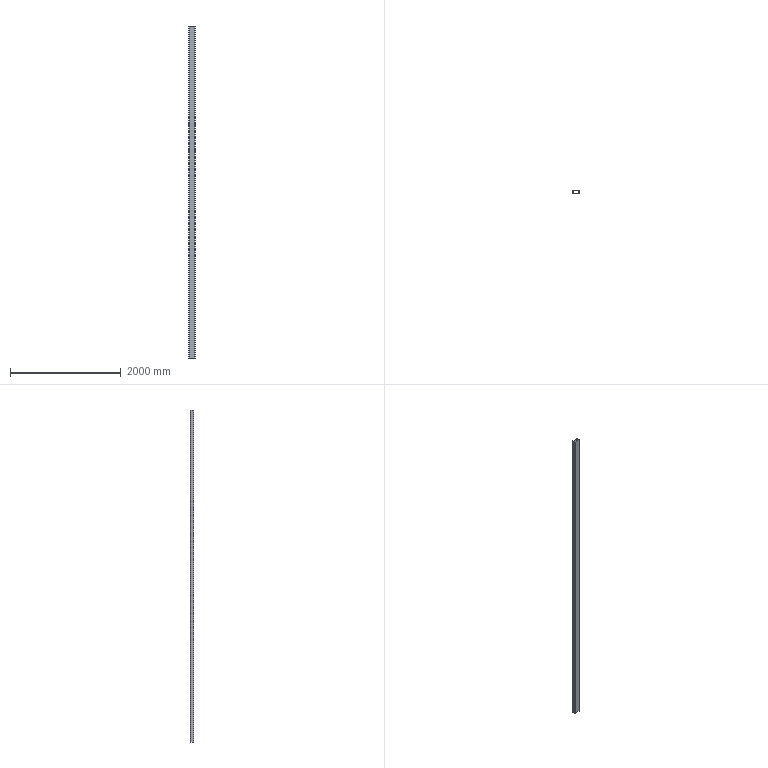Part | SolidWorks | features Extrusion 1 | 1 solid | 18 faces | box 120 x 60 x 6000 mm | volume 9813717 mm3 | plane 10 | cylinder 8 | commonest cylinder face diameters 10 x4 20 x4
STEP:
#1=CARTESIAN_POINT('',(110.,0.,6000.));
#2=VERTEX_POINT('',#1);
#3=CARTESIAN_POINT('',(120.,10.,6000.));
#4=VERTEX_POINT('',#3);
#5=CARTESIAN_POINT('',(110.,10.,6000.));
#6=DIRECTION('',(0.,0.,1.));
#7=DIRECTION('',(-1.,0.,0.));
#8=AXIS2_PLACEMENT_3D('',#5,#6,#7);
#9=CIRCLE('',#8,10.);
#10=EDGE_CURVE('',#2,#4,#9,.T.);
#11=ORIENTED_EDGE('',*,*,#10,.T.);
#12=CARTESIAN_POINT('',(120.,50.,6000.));
#13=VERTEX_POINT('',#12);
#14=CARTESIAN_POINT('',(120.,10.,6000.));
#15=DIRECTION('',(0.,1.,0.));
#16=VECTOR('',#15,1000.);
#17=LINE('',#14,#16);
#18=EDGE_CURVE('',#4,#13,#17,.T.);
#19=ORIENTED_EDGE('',*,*,#18,.T.);
#20=CARTESIAN_POINT('',(110.,60.,6000.));
#21=VERTEX_POINT('',#20);
#22=CARTESIAN_POINT('',(110.,50.,6000.));
#23=DIRECTION('',(0.,0.,1.));
#24=DIRECTION('',(1.,0.,0.));
#25=AXIS2_PLACEMENT_3D('',#22,#23,#24);
#26=CIRCLE('',#25,10.);
#27=EDGE_CURVE('',#13,#21,#26,.T.);
#28=ORIENTED_EDGE('',*,*,#27,.T.);
#29=CARTESIAN_POINT('',(10.,60.,6000.));
#30=VERTEX_POINT('',#29);
#31=CARTESIAN_POINT('',(10.,60.,6000.));
#32=DIRECTION('',(-1.,0.,0.));
#33=VECTOR('',#32,1000.);
#34=LINE('',#31,#33);
#35=EDGE_CURVE('',#21,#30,#34,.T.);
#36=ORIENTED_EDGE('',*,*,#35,.T.);
#37=CARTESIAN_POINT('',(0.,50.,6000.));
#38=VERTEX_POINT('',#37);
#39=CARTESIAN_POINT('',(10.,50.,6000.));
#40=DIRECTION('',(0.,0.,1.));
#41=DIRECTION('',(-1.,0.,0.));
#42=AXIS2_PLACEMENT_3D('',#39,#40,#41);
#43=CIRCLE('',#42,10.);
#44=EDGE_CURVE('',#30,#38,#43,.T.);
#45=ORIENTED_EDGE('',*,*,#44,.T.);
#46=CARTESIAN_POINT('',(0.,10.,6000.));
#47=VERTEX_POINT('',#46);
#48=CARTESIAN_POINT('',(0.,10.,6000.));
#49=DIRECTION('',(0.,-1.,0.));
#50=VECTOR('',#49,1000.);
#51=LINE('',#48,#50);
#52=EDGE_CURVE('',#38,#47,#51,.T.);
#53=ORIENTED_EDGE('',*,*,#52,.T.);
#54=CARTESIAN_POINT('',(10.,0.,6000.));
#55=VERTEX_POINT('',#54);
#56=CARTESIAN_POINT('',(10.,10.,6000.));
#57=DIRECTION('',(0.,0.,1.));
#58=DIRECTION('',(-1.,0.,0.));
#59=AXIS2_PLACEMENT_3D('',#56,#57,#58);
#60=CIRCLE('',#59,10.);
#61=EDGE_CURVE('',#47,#55,#60,.T.);
#62=ORIENTED_EDGE('',*,*,#61,.T.);
#63=CARTESIAN_POINT('',(10.,0.,6000.));
#64=DIRECTION('',(1.,0.,0.));
#65=VECTOR('',#64,1000.);
#66=LINE('',#63,#65);
#67=EDGE_CURVE('',#55,#2,#66,.T.);
#68=ORIENTED_EDGE('',*,*,#67,.T.);
#69=EDGE_LOOP('',(#11,#19,#28,#36,#45,#53,#62,#68));
#70=FACE_OUTER_BOUND('',#69,.T.);
#71=CARTESIAN_POINT('',(10.,55.,6000.));
#72=VERTEX_POINT('',#71);
#73=CARTESIAN_POINT('',(5.,50.,6000.));
#74=VERTEX_POINT('',#73);
#75=CARTESIAN_POINT('',(10.,50.,6000.));
#76=DIRECTION('',(0.,0.,1.));
#77=DIRECTION('',(-1.,0.,0.));
#78=AXIS2_PLACEMENT_3D('',#75,#76,#77);
#79=CIRCLE('',#78,5.);
#80=EDGE_CURVE('',#72,#74,#79,.T.);
#81=ORIENTED_EDGE('',*,*,#80,.F.);
#82=CARTESIAN_POINT('',(110.,55.,6000.));
#83=VERTEX_POINT('',#82);
#84=CARTESIAN_POINT('',(10.,55.,6000.));
#85=DIRECTION('',(-1.,0.,0.));
#86=VECTOR('',#85,1000.);
#87=LINE('',#84,#86);
#88=EDGE_CURVE('',#83,#72,#87,.T.);
#89=ORIENTED_EDGE('',*,*,#88,.F.);
#90=CARTESIAN_POINT('',(115.,50.,6000.));
#91=VERTEX_POINT('',#90);
#92=CARTESIAN_POINT('',(110.,50.,6000.));
#93=DIRECTION('',(0.,0.,1.));
#94=DIRECTION('',(1.,0.,0.));
#95=AXIS2_PLACEMENT_3D('',#92,#93,#94);
#96=CIRCLE('',#95,5.);
#97=EDGE_CURVE('',#91,#83,#96,.T.);
#98=ORIENTED_EDGE('',*,*,#97,.F.);
#99=CARTESIAN_POINT('',(115.,10.,6000.));
#100=VERTEX_POINT('',#99);
#101=CARTESIAN_POINT('',(115.,10.,6000.));
#102=DIRECTION('',(0.,1.,0.));
#103=VECTOR('',#102,1000.);
#104=LINE('',#101,#103);
#105=EDGE_CURVE('',#100,#91,#104,.T.);
#106=ORIENTED_EDGE('',*,*,#105,.F.);
#107=CARTESIAN_POINT('',(110.,5.,6000.));
#108=VERTEX_POINT('',#107);
#109=CARTESIAN_POINT('',(110.,10.,6000.));
#110=DIRECTION('',(0.,0.,1.));
#111=DIRECTION('',(-1.,0.,0.));
#112=AXIS2_PLACEMENT_3D('',#109,#110,#111);
#113=CIRCLE('',#112,5.);
#114=EDGE_CURVE('',#108,#100,#113,.T.);
#115=ORIENTED_EDGE('',*,*,#114,.F.);
#116=CARTESIAN_POINT('',(10.,5.,6000.));
#117=VERTEX_POINT('',#116);
#118=CARTESIAN_POINT('',(10.,5.,6000.));
#119=DIRECTION('',(1.,0.,0.));
#120=VECTOR('',#119,1000.);
#121=LINE('',#118,#120);
#122=EDGE_CURVE('',#117,#108,#121,.T.);
#123=ORIENTED_EDGE('',*,*,#122,.F.);
#124=CARTESIAN_POINT('',(5.,10.,6000.));
#125=VERTEX_POINT('',#124);
#126=CARTESIAN_POINT('',(10.,10.,6000.));
#127=DIRECTION('',(0.,0.,1.));
#128=DIRECTION('',(-1.,0.,0.));
#129=AXIS2_PLACEMENT_3D('',#126,#127,#128);
#130=CIRCLE('',#129,5.);
#131=EDGE_CURVE('',#125,#117,#130,.T.);
#132=ORIENTED_EDGE('',*,*,#131,.F.);
#133=CARTESIAN_POINT('',(5.,10.,6000.));
#134=DIRECTION('',(0.,-1.,0.));
#135=VECTOR('',#134,1000.);
#136=LINE('',#133,#135);
#137=EDGE_CURVE('',#74,#125,#136,.T.);
#138=ORIENTED_EDGE('',*,*,#137,.F.);
#139=EDGE_LOOP('',(#81,#89,#98,#106,#115,#123,#132,#138));
#140=FACE_BOUND('',#139,.T.);
#141=CARTESIAN_POINT('',(110.,10.,6000.));
#142=DIRECTION('',(0.,0.,-1.));
#143=DIRECTION('',(-1.,0.,0.));
#144=AXIS2_PLACEMENT_3D('',#141,#142,#143);
#145=PLANE('',#144);
#146=ADVANCED_FACE('',(#70,#140),#145,.F.);
#147=CARTESIAN_POINT('',(110.,0.,0.));
#148=VERTEX_POINT('',#147);
#149=CARTESIAN_POINT('',(120.,10.,0.));
#150=VERTEX_POINT('',#149);
#151=CARTESIAN_POINT('',(110.,10.,0.));
#152=DIRECTION('',(0.,0.,1.));
#153=DIRECTION('',(-1.,0.,0.));
#154=AXIS2_PLACEMENT_3D('',#151,#152,#153);
#155=CIRCLE('',#154,10.);
#156=EDGE_CURVE('',#148,#150,#155,.T.);
#157=ORIENTED_EDGE('',*,*,#156,.F.);
#158=CARTESIAN_POINT('',(10.,0.,0.));
#159=VERTEX_POINT('',#158);
#160=CARTESIAN_POINT('',(10.,0.,0.));
#161=DIRECTION('',(1.,0.,0.));
#162=VECTOR('',#161,1000.);
#163=LINE('',#160,#162);
#164=EDGE_CURVE('',#159,#148,#163,.T.);
#165=ORIENTED_EDGE('',*,*,#164,.F.);
#166=CARTESIAN_POINT('',(0.,10.,0.));
#167=VERTEX_POINT('',#166);
#168=CARTESIAN_POINT('',(10.,10.,0.));
#169=DIRECTION('',(0.,0.,1.));
#170=DIRECTION('',(-1.,0.,0.));
#171=AXIS2_PLACEMENT_3D('',#168,#169,#170);
#172=CIRCLE('',#171,10.);
#173=EDGE_CURVE('',#167,#159,#172,.T.);
#174=ORIENTED_EDGE('',*,*,#173,.F.);
#175=CARTESIAN_POINT('',(0.,50.,0.));
#176=VERTEX_POINT('',#175);
#177=CARTESIAN_POINT('',(0.,10.,0.));
#178=DIRECTION('',(0.,-1.,0.));
#179=VECTOR('',#178,1000.);
#180=LINE('',#177,#179);
#181=EDGE_CURVE('',#176,#167,#180,.T.);
#182=ORIENTED_EDGE('',*,*,#181,.F.);
#183=CARTESIAN_POINT('',(10.,60.,0.));
#184=VERTEX_POINT('',#183);
#185=CARTESIAN_POINT('',(10.,50.,0.));
#186=DIRECTION('',(0.,0.,1.));
#187=DIRECTION('',(-1.,0.,0.));
#188=AXIS2_PLACEMENT_3D('',#185,#186,#187);
#189=CIRCLE('',#188,10.);
#190=EDGE_CURVE('',#184,#176,#189,.T.);
#191=ORIENTED_EDGE('',*,*,#190,.F.);
#192=CARTESIAN_POINT('',(110.,60.,0.));
#193=VERTEX_POINT('',#192);
#194=CARTESIAN_POINT('',(10.,60.,0.));
#195=DIRECTION('',(-1.,0.,0.));
#196=VECTOR('',#195,1000.);
#197=LINE('',#194,#196);
#198=EDGE_CURVE('',#193,#184,#197,.T.);
#199=ORIENTED_EDGE('',*,*,#198,.F.);
#200=CARTESIAN_POINT('',(120.,50.,0.));
#201=VERTEX_POINT('',#200);
#202=CARTESIAN_POINT('',(110.,50.,0.));
#203=DIRECTION('',(0.,0.,1.));
#204=DIRECTION('',(1.,0.,0.));
#205=AXIS2_PLACEMENT_3D('',#202,#203,#204);
#206=CIRCLE('',#205,10.);
#207=EDGE_CURVE('',#201,#193,#206,.T.);
#208=ORIENTED_EDGE('',*,*,#207,.F.);
#209=CARTESIAN_POINT('',(120.,10.,0.));
#210=DIRECTION('',(0.,1.,0.));
#211=VECTOR('',#210,1000.);
#212=LINE('',#209,#211);
#213=EDGE_CURVE('',#150,#201,#212,.T.);
#214=ORIENTED_EDGE('',*,*,#213,.F.);
#215=EDGE_LOOP('',(#157,#165,#174,#182,#191,#199,#208,#214));
#216=FACE_OUTER_BOUND('',#215,.T.);
#217=CARTESIAN_POINT('',(110.,55.,0.));
#218=VERTEX_POINT('',#217);
#219=CARTESIAN_POINT('',(10.,55.,0.));
#220=VERTEX_POINT('',#219);
#221=CARTESIAN_POINT('',(10.,55.,0.));
#222=DIRECTION('',(-1.,0.,0.));
#223=VECTOR('',#222,1000.);
#224=LINE('',#221,#223);
#225=EDGE_CURVE('',#218,#220,#224,.T.);
#226=ORIENTED_EDGE('',*,*,#225,.T.);
#227=CARTESIAN_POINT('',(5.,50.,0.));
#228=VERTEX_POINT('',#227);
#229=CARTESIAN_POINT('',(10.,50.,0.));
#230=DIRECTION('',(0.,0.,1.));
#231=DIRECTION('',(-1.,0.,0.));
#232=AXIS2_PLACEMENT_3D('',#229,#230,#231);
#233=CIRCLE('',#232,5.);
#234=EDGE_CURVE('',#220,#228,#233,.T.);
#235=ORIENTED_EDGE('',*,*,#234,.T.);
#236=CARTESIAN_POINT('',(5.,10.,0.));
#237=VERTEX_POINT('',#236);
#238=CARTESIAN_POINT('',(5.,10.,0.));
#239=DIRECTION('',(0.,-1.,0.));
#240=VECTOR('',#239,1000.);
#241=LINE('',#238,#240);
#242=EDGE_CURVE('',#228,#237,#241,.T.);
#243=ORIENTED_EDGE('',*,*,#242,.T.);
#244=CARTESIAN_POINT('',(10.,5.,0.));
#245=VERTEX_POINT('',#244);
#246=CARTESIAN_POINT('',(10.,10.,0.));
#247=DIRECTION('',(0.,0.,1.));
#248=DIRECTION('',(-1.,0.,0.));
#249=AXIS2_PLACEMENT_3D('',#246,#247,#248);
#250=CIRCLE('',#249,5.);
#251=EDGE_CURVE('',#237,#245,#250,.T.);
#252=ORIENTED_EDGE('',*,*,#251,.T.);
#253=CARTESIAN_POINT('',(110.,5.,0.));
#254=VERTEX_POINT('',#253);
#255=CARTESIAN_POINT('',(10.,5.,0.));
#256=DIRECTION('',(1.,0.,0.));
#257=VECTOR('',#256,1000.);
#258=LINE('',#255,#257);
#259=EDGE_CURVE('',#245,#254,#258,.T.);
#260=ORIENTED_EDGE('',*,*,#259,.T.);
#261=CARTESIAN_POINT('',(115.,10.,0.));
#262=VERTEX_POINT('',#261);
#263=CARTESIAN_POINT('',(110.,10.,0.));
#264=DIRECTION('',(0.,0.,1.));
#265=DIRECTION('',(-1.,0.,0.));
#266=AXIS2_PLACEMENT_3D('',#263,#264,#265);
#267=CIRCLE('',#266,5.);
#268=EDGE_CURVE('',#254,#262,#267,.T.);
#269=ORIENTED_EDGE('',*,*,#268,.T.);
#270=CARTESIAN_POINT('',(115.,50.,0.));
#271=VERTEX_POINT('',#270);
#272=CARTESIAN_POINT('',(115.,10.,0.));
#273=DIRECTION('',(0.,1.,0.));
#274=VECTOR('',#273,1000.);
#275=LINE('',#272,#274);
#276=EDGE_CURVE('',#262,#271,#275,.T.);
#277=ORIENTED_EDGE('',*,*,#276,.T.);
#278=CARTESIAN_POINT('',(110.,50.,0.));
#279=DIRECTION('',(0.,0.,1.));
#280=DIRECTION('',(1.,0.,0.));
#281=AXIS2_PLACEMENT_3D('',#278,#279,#280);
#282=CIRCLE('',#281,5.);
#283=EDGE_CURVE('',#271,#218,#282,.T.);
#284=ORIENTED_EDGE('',*,*,#283,.T.);
#285=EDGE_LOOP('',(#226,#235,#243,#252,#260,#269,#277,#284));
#286=FACE_BOUND('',#285,.T.);
#287=CARTESIAN_POINT('',(110.,10.,0.));
#288=DIRECTION('',(0.,0.,-1.));
#289=DIRECTION('',(-1.,0.,0.));
#290=AXIS2_PLACEMENT_3D('',#287,#288,#289);
#291=PLANE('',#290);
#292=ADVANCED_FACE('',(#216,#286),#291,.T.);
#293=ORIENTED_EDGE('',*,*,#156,.T.);
#294=CARTESIAN_POINT('',(120.,10.,6000.));
#295=DIRECTION('',(0.,0.,-1.));
#296=VECTOR('',#295,1000.);
#297=LINE('',#294,#296);
#298=EDGE_CURVE('',#4,#150,#297,.T.);
#299=ORIENTED_EDGE('',*,*,#298,.F.);
#300=ORIENTED_EDGE('',*,*,#10,.F.);
#301=CARTESIAN_POINT('',(110.,0.,6000.));
#302=DIRECTION('',(0.,0.,-1.));
#303=VECTOR('',#302,1000.);
#304=LINE('',#301,#303);
#305=EDGE_CURVE('',#2,#148,#304,.T.);
#306=ORIENTED_EDGE('',*,*,#305,.T.);
#307=EDGE_LOOP('',(#293,#299,#300,#306));
#308=FACE_OUTER_BOUND('',#307,.T.);
#309=CARTESIAN_POINT('',(110.,10.,6000.));
#310=DIRECTION('',(0.,0.,-1.));
#311=DIRECTION('',(-1.,0.,0.));
#312=AXIS2_PLACEMENT_3D('',#309,#310,#311);
#313=CYLINDRICAL_SURFACE('',#312,10.);
#314=ADVANCED_FACE('',(#308),#313,.T.);
#315=ORIENTED_EDGE('',*,*,#213,.T.);
#316=CARTESIAN_POINT('',(120.,50.,6000.));
#317=DIRECTION('',(0.,0.,-1.));
#318=VECTOR('',#317,1000.);
#319=LINE('',#316,#318);
#320=EDGE_CURVE('',#13,#201,#319,.T.);
#321=ORIENTED_EDGE('',*,*,#320,.F.);
#322=ORIENTED_EDGE('',*,*,#18,.F.);
#323=ORIENTED_EDGE('',*,*,#298,.T.);
#324=EDGE_LOOP('',(#315,#321,#322,#323));
#325=FACE_OUTER_BOUND('',#324,.T.);
#326=CARTESIAN_POINT('',(120.,10.,6000.));
#327=DIRECTION('',(-1.,0.,0.));
#328=DIRECTION('',(0.,-1.,0.));
#329=AXIS2_PLACEMENT_3D('',#326,#327,#328);
#330=PLANE('',#329);
#331=ADVANCED_FACE('',(#325),#330,.F.);
#332=ORIENTED_EDGE('',*,*,#207,.T.);
#333=CARTESIAN_POINT('',(110.,60.,6000.));
#334=DIRECTION('',(0.,0.,-1.));
#335=VECTOR('',#334,1000.);
#336=LINE('',#333,#335);
#337=EDGE_CURVE('',#21,#193,#336,.T.);
#338=ORIENTED_EDGE('',*,*,#337,.F.);
#339=ORIENTED_EDGE('',*,*,#27,.F.);
#340=ORIENTED_EDGE('',*,*,#320,.T.);
#341=EDGE_LOOP('',(#332,#338,#339,#340));
#342=FACE_OUTER_BOUND('',#341,.T.);
#343=CARTESIAN_POINT('',(110.,50.,6000.));
#344=DIRECTION('',(0.,0.,-1.));
#345=DIRECTION('',(-1.,0.,0.));
#346=AXIS2_PLACEMENT_3D('',#343,#344,#345);
#347=CYLINDRICAL_SURFACE('',#346,10.);
#348=ADVANCED_FACE('',(#342),#347,.T.);
#349=ORIENTED_EDGE('',*,*,#198,.T.);
#350=CARTESIAN_POINT('',(10.,60.,6000.));
#351=DIRECTION('',(0.,0.,-1.));
#352=VECTOR('',#351,1000.);
#353=LINE('',#350,#352);
#354=EDGE_CURVE('',#30,#184,#353,.T.);
#355=ORIENTED_EDGE('',*,*,#354,.F.);
#356=ORIENTED_EDGE('',*,*,#35,.F.);
#357=ORIENTED_EDGE('',*,*,#337,.T.);
#358=EDGE_LOOP('',(#349,#355,#356,#357));
#359=FACE_OUTER_BOUND('',#358,.T.);
#360=CARTESIAN_POINT('',(10.,60.,6000.));
#361=DIRECTION('',(0.,-1.,0.));
#362=DIRECTION('',(0.,0.,-1.));
#363=AXIS2_PLACEMENT_3D('',#360,#361,#362);
#364=PLANE('',#363);
#365=ADVANCED_FACE('',(#359),#364,.F.);
#366=ORIENTED_EDGE('',*,*,#190,.T.);
#367=CARTESIAN_POINT('',(0.,50.,6000.));
#368=DIRECTION('',(0.,0.,-1.));
#369=VECTOR('',#368,1000.);
#370=LINE('',#367,#369);
#371=EDGE_CURVE('',#38,#176,#370,.T.);
#372=ORIENTED_EDGE('',*,*,#371,.F.);
#373=ORIENTED_EDGE('',*,*,#44,.F.);
#374=ORIENTED_EDGE('',*,*,#354,.T.);
#375=EDGE_LOOP('',(#366,#372,#373,#374));
#376=FACE_OUTER_BOUND('',#375,.T.);
#377=CARTESIAN_POINT('',(10.,50.,6000.));
#378=DIRECTION('',(0.,0.,-1.));
#379=DIRECTION('',(-1.,0.,0.));
#380=AXIS2_PLACEMENT_3D('',#377,#378,#379);
#381=CYLINDRICAL_SURFACE('',#380,10.);
#382=ADVANCED_FACE('',(#376),#381,.T.);
#383=ORIENTED_EDGE('',*,*,#181,.T.);
#384=CARTESIAN_POINT('',(0.,10.,6000.));
#385=DIRECTION('',(0.,0.,-1.));
#386=VECTOR('',#385,1000.);
#387=LINE('',#384,#386);
#388=EDGE_CURVE('',#47,#167,#387,.T.);
#389=ORIENTED_EDGE('',*,*,#388,.F.);
#390=ORIENTED_EDGE('',*,*,#52,.F.);
#391=ORIENTED_EDGE('',*,*,#371,.T.);
#392=EDGE_LOOP('',(#383,#389,#390,#391));
#393=FACE_OUTER_BOUND('',#392,.T.);
#394=CARTESIAN_POINT('',(0.,10.,6000.));
#395=DIRECTION('',(1.,0.,0.));
#396=DIRECTION('',(0.,1.,0.));
#397=AXIS2_PLACEMENT_3D('',#394,#395,#396);
#398=PLANE('',#397);
#399=ADVANCED_FACE('',(#393),#398,.F.);
#400=ORIENTED_EDGE('',*,*,#173,.T.);
#401=CARTESIAN_POINT('',(10.,0.,6000.));
#402=DIRECTION('',(0.,0.,-1.));
#403=VECTOR('',#402,1000.);
#404=LINE('',#401,#403);
#405=EDGE_CURVE('',#55,#159,#404,.T.);
#406=ORIENTED_EDGE('',*,*,#405,.F.);
#407=ORIENTED_EDGE('',*,*,#61,.F.);
#408=ORIENTED_EDGE('',*,*,#388,.T.);
#409=EDGE_LOOP('',(#400,#406,#407,#408));
#410=FACE_OUTER_BOUND('',#409,.T.);
#411=CARTESIAN_POINT('',(10.,10.,6000.));
#412=DIRECTION('',(0.,0.,-1.));
#413=DIRECTION('',(-1.,0.,0.));
#414=AXIS2_PLACEMENT_3D('',#411,#412,#413);
#415=CYLINDRICAL_SURFACE('',#414,10.);
#416=ADVANCED_FACE('',(#410),#415,.T.);
#417=ORIENTED_EDGE('',*,*,#164,.T.);
#418=ORIENTED_EDGE('',*,*,#305,.F.);
#419=ORIENTED_EDGE('',*,*,#67,.F.);
#420=ORIENTED_EDGE('',*,*,#405,.T.);
#421=EDGE_LOOP('',(#417,#418,#419,#420));
#422=FACE_OUTER_BOUND('',#421,.T.);
#423=CARTESIAN_POINT('',(10.,0.,6000.));
#424=DIRECTION('',(0.,1.,0.));
#425=DIRECTION('',(0.,0.,1.));
#426=AXIS2_PLACEMENT_3D('',#423,#424,#425);
#427=PLANE('',#426);
#428=ADVANCED_FACE('',(#422),#427,.F.);
#429=ORIENTED_EDGE('',*,*,#234,.F.);
#430=CARTESIAN_POINT('',(10.,55.,6000.));
#431=DIRECTION('',(0.,0.,-1.));
#432=VECTOR('',#431,1000.);
#433=LINE('',#430,#432);
#434=EDGE_CURVE('',#72,#220,#433,.T.);
#435=ORIENTED_EDGE('',*,*,#434,.F.);
#436=ORIENTED_EDGE('',*,*,#80,.T.);
#437=CARTESIAN_POINT('',(5.,50.,6000.));
#438=DIRECTION('',(0.,0.,-1.));
#439=VECTOR('',#438,1000.);
#440=LINE('',#437,#439);
#441=EDGE_CURVE('',#74,#228,#440,.T.);
#442=ORIENTED_EDGE('',*,*,#441,.T.);
#443=EDGE_LOOP('',(#429,#435,#436,#442));
#444=FACE_OUTER_BOUND('',#443,.T.);
#445=CARTESIAN_POINT('',(10.,50.,6000.));
#446=DIRECTION('',(0.,0.,-1.));
#447=DIRECTION('',(-1.,0.,0.));
#448=AXIS2_PLACEMENT_3D('',#445,#446,#447);
#449=CYLINDRICAL_SURFACE('',#448,5.);
#450=ADVANCED_FACE('',(#444),#449,.F.);
#451=ORIENTED_EDGE('',*,*,#242,.F.);
#452=ORIENTED_EDGE('',*,*,#441,.F.);
#453=ORIENTED_EDGE('',*,*,#137,.T.);
#454=CARTESIAN_POINT('',(5.,10.,6000.));
#455=DIRECTION('',(0.,0.,-1.));
#456=VECTOR('',#455,1000.);
#457=LINE('',#454,#456);
#458=EDGE_CURVE('',#125,#237,#457,.T.);
#459=ORIENTED_EDGE('',*,*,#458,.T.);
#460=EDGE_LOOP('',(#451,#452,#453,#459));
#461=FACE_OUTER_BOUND('',#460,.T.);
#462=CARTESIAN_POINT('',(5.,10.,6000.));
#463=DIRECTION('',(1.,0.,0.));
#464=DIRECTION('',(0.,1.,0.));
#465=AXIS2_PLACEMENT_3D('',#462,#463,#464);
#466=PLANE('',#465);
#467=ADVANCED_FACE('',(#461),#466,.T.);
#468=ORIENTED_EDGE('',*,*,#251,.F.);
#469=ORIENTED_EDGE('',*,*,#458,.F.);
#470=ORIENTED_EDGE('',*,*,#131,.T.);
#471=CARTESIAN_POINT('',(10.,5.,6000.));
#472=DIRECTION('',(0.,0.,-1.));
#473=VECTOR('',#472,1000.);
#474=LINE('',#471,#473);
#475=EDGE_CURVE('',#117,#245,#474,.T.);
#476=ORIENTED_EDGE('',*,*,#475,.T.);
#477=EDGE_LOOP('',(#468,#469,#470,#476));
#478=FACE_OUTER_BOUND('',#477,.T.);
#479=CARTESIAN_POINT('',(10.,10.,6000.));
#480=DIRECTION('',(0.,0.,-1.));
#481=DIRECTION('',(-1.,0.,0.));
#482=AXIS2_PLACEMENT_3D('',#479,#480,#481);
#483=CYLINDRICAL_SURFACE('',#482,5.);
#484=ADVANCED_FACE('',(#478),#483,.F.);
#485=ORIENTED_EDGE('',*,*,#259,.F.);
#486=ORIENTED_EDGE('',*,*,#475,.F.);
#487=ORIENTED_EDGE('',*,*,#122,.T.);
#488=CARTESIAN_POINT('',(110.,5.,6000.));
#489=DIRECTION('',(0.,0.,-1.));
#490=VECTOR('',#489,1000.);
#491=LINE('',#488,#490);
#492=EDGE_CURVE('',#108,#254,#491,.T.);
#493=ORIENTED_EDGE('',*,*,#492,.T.);
#494=EDGE_LOOP('',(#485,#486,#487,#493));
#495=FACE_OUTER_BOUND('',#494,.T.);
#496=CARTESIAN_POINT('',(10.,5.,6000.));
#497=DIRECTION('',(0.,1.,0.));
#498=DIRECTION('',(0.,0.,1.));
#499=AXIS2_PLACEMENT_3D('',#496,#497,#498);
#500=PLANE('',#499);
#501=ADVANCED_FACE('',(#495),#500,.T.);
#502=ORIENTED_EDGE('',*,*,#268,.F.);
#503=ORIENTED_EDGE('',*,*,#492,.F.);
#504=ORIENTED_EDGE('',*,*,#114,.T.);
#505=CARTESIAN_POINT('',(115.,10.,6000.));
#506=DIRECTION('',(0.,0.,-1.));
#507=VECTOR('',#506,1000.);
#508=LINE('',#505,#507);
#509=EDGE_CURVE('',#100,#262,#508,.T.);
#510=ORIENTED_EDGE('',*,*,#509,.T.);
#511=EDGE_LOOP('',(#502,#503,#504,#510));
#512=FACE_OUTER_BOUND('',#511,.T.);
#513=CARTESIAN_POINT('',(110.,10.,6000.));
#514=DIRECTION('',(0.,0.,-1.));
#515=DIRECTION('',(-1.,0.,0.));
#516=AXIS2_PLACEMENT_3D('',#513,#514,#515);
#517=CYLINDRICAL_SURFACE('',#516,5.);
#518=ADVANCED_FACE('',(#512),#517,.F.);
#519=ORIENTED_EDGE('',*,*,#276,.F.);
#520=ORIENTED_EDGE('',*,*,#509,.F.);
#521=ORIENTED_EDGE('',*,*,#105,.T.);
#522=CARTESIAN_POINT('',(115.,50.,6000.));
#523=DIRECTION('',(0.,0.,-1.));
#524=VECTOR('',#523,1000.);
#525=LINE('',#522,#524);
#526=EDGE_CURVE('',#91,#271,#525,.T.);
#527=ORIENTED_EDGE('',*,*,#526,.T.);
#528=EDGE_LOOP('',(#519,#520,#521,#527));
#529=FACE_OUTER_BOUND('',#528,.T.);
#530=CARTESIAN_POINT('',(115.,10.,6000.));
#531=DIRECTION('',(-1.,0.,0.));
#532=DIRECTION('',(0.,0.,1.));
#533=AXIS2_PLACEMENT_3D('',#530,#531,#532);
#534=PLANE('',#533);
#535=ADVANCED_FACE('',(#529),#534,.T.);
#536=ORIENTED_EDGE('',*,*,#283,.F.);
#537=ORIENTED_EDGE('',*,*,#526,.F.);
#538=ORIENTED_EDGE('',*,*,#97,.T.);
#539=CARTESIAN_POINT('',(110.,55.,6000.));
#540=DIRECTION('',(0.,0.,-1.));
#541=VECTOR('',#540,1000.);
#542=LINE('',#539,#541);
#543=EDGE_CURVE('',#83,#218,#542,.T.);
#544=ORIENTED_EDGE('',*,*,#543,.T.);
#545=EDGE_LOOP('',(#536,#537,#538,#544));
#546=FACE_OUTER_BOUND('',#545,.T.);
#547=CARTESIAN_POINT('',(110.,50.,6000.));
#548=DIRECTION('',(0.,0.,-1.));
#549=DIRECTION('',(-1.,0.,0.));
#550=AXIS2_PLACEMENT_3D('',#547,#548,#549);
#551=CYLINDRICAL_SURFACE('',#550,5.);
#552=ADVANCED_FACE('',(#546),#551,.F.);
#553=ORIENTED_EDGE('',*,*,#225,.F.);
#554=ORIENTED_EDGE('',*,*,#543,.F.);
#555=ORIENTED_EDGE('',*,*,#88,.T.);
#556=ORIENTED_EDGE('',*,*,#434,.T.);
#557=EDGE_LOOP('',(#553,#554,#555,#556));
#558=FACE_OUTER_BOUND('',#557,.T.);
#559=CARTESIAN_POINT('',(10.,55.,6000.));
#560=DIRECTION('',(0.,-1.,0.));
#561=DIRECTION('',(0.,0.,-1.));
#562=AXIS2_PLACEMENT_3D('',#559,#560,#561);
#563=PLANE('',#562);
#564=ADVANCED_FACE('',(#558),#563,.T.);
#565=CLOSED_SHELL('',(#146,#292,#314,#331,#348,#365,#382,#399,#416,#428,#450,#467,#484,#501,#518,#535,#552,#564));
#566=MANIFOLD_SOLID_BREP('',#565);
#567=CARTESIAN_POINT('',(0.,0.,0.));
#568=DIRECTION('',(0.,0.,1.));
#569=DIRECTION('',(1.,0.,0.));
#570=AXIS2_PLACEMENT_3D('',#567,#568,#569);
#571=(LENGTH_UNIT()NAMED_UNIT(*)SI_UNIT(.MILLI.,.METRE.));
#572=UNCERTAINTY_MEASURE_WITH_UNIT(LENGTH_MEASURE(0.00001),#571,'','');
#573=(NAMED_UNIT(*)PLANE_ANGLE_UNIT()SI_UNIT($,.RADIAN.));
#574=(NAMED_UNIT(*)SI_UNIT($,.STERADIAN.)SOLID_ANGLE_UNIT());
#575=(GEOMETRIC_REPRESENTATION_CONTEXT(3)GLOBAL_UNCERTAINTY_ASSIGNED_CONTEXT((#572))GLOBAL_UNIT_ASSIGNED_CONTEXT((#571,#573,#574))REPRESENTATION_CONTEXT('',''));
#576=ADVANCED_BREP_SHAPE_REPRESENTATION('',(#566,#570),#575);